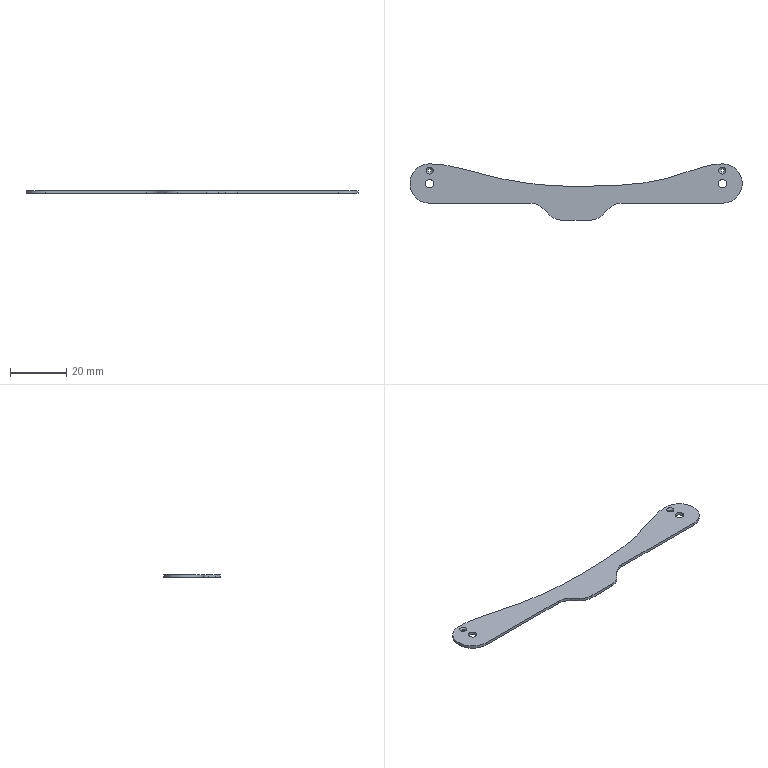Part | NX | features BREP 1, DATUM_CSYS 1, SCALE 1 | 1 solid | 23 faces | box 118 x 20 x 1 mm | volume 1195 mm3 | cylinder 11 | plane 8 | cone 2 | spline 2 | commonest cylinder face diameters 12 x5 1.32 x2 3 x2 14 x2
STEP:
#1=CARTESIAN_POINT('',(-50.74,4.6,1.));
#2=VERTEX_POINT('',#1);
#3=CARTESIAN_POINT('',(-52.,4.6,1.));
#4=DIRECTION('',(0.,0.,1.));
#5=DIRECTION('',(1.,0.,0.));
#6=AXIS2_PLACEMENT_3D('',#3,#4,#5);
#7=CIRCLE('',#6,1.26);
#8=EDGE_CURVE('',#2,#2,#7,.T.);
#9=ORIENTED_EDGE('',*,*,#8,.T.);
#10=EDGE_LOOP('',(#9));
#11=FACE_BOUND('',#10,.T.);
#12=CARTESIAN_POINT('',(-51.34,4.6,0.4));
#13=VERTEX_POINT('',#12);
#14=CARTESIAN_POINT('',(-52.,4.6,0.4));
#15=DIRECTION('',(0.,0.,1.));
#16=DIRECTION('',(1.,0.,0.));
#17=AXIS2_PLACEMENT_3D('',#14,#15,#16);
#18=CIRCLE('',#17,0.66);
#19=EDGE_CURVE('',#13,#13,#18,.T.);
#20=ORIENTED_EDGE('',*,*,#19,.F.);
#21=EDGE_LOOP('',(#20));
#22=FACE_BOUND('',#21,.T.);
#23=CARTESIAN_POINT('',(-52.,4.6,1.));
#24=DIRECTION('',(0.,0.,1.));
#25=DIRECTION('',(1.,0.,0.));
#26=AXIS2_PLACEMENT_3D('',#23,#24,#25);
#27=CONICAL_SURFACE('',#26,1.26,0.7854);
#28=ADVANCED_FACE('',(#11,#22),#27,.F.);
#29=ORIENTED_EDGE('',*,*,#19,.T.);
#30=EDGE_LOOP('',(#29));
#31=FACE_BOUND('',#30,.T.);
#32=CARTESIAN_POINT('',(-51.34,4.6,0.));
#33=VERTEX_POINT('',#32);
#34=CARTESIAN_POINT('',(-52.,4.6,0.));
#35=DIRECTION('',(0.,0.,1.));
#36=DIRECTION('',(1.,0.,0.));
#37=AXIS2_PLACEMENT_3D('',#34,#35,#36);
#38=CIRCLE('',#37,0.66);
#39=EDGE_CURVE('',#33,#33,#38,.T.);
#40=ORIENTED_EDGE('',*,*,#39,.F.);
#41=EDGE_LOOP('',(#40));
#42=FACE_BOUND('',#41,.T.);
#43=CARTESIAN_POINT('',(-52.,4.6,1.));
#44=DIRECTION('',(0.,0.,1.));
#45=DIRECTION('',(1.,0.,0.));
#46=AXIS2_PLACEMENT_3D('',#43,#44,#45);
#47=CYLINDRICAL_SURFACE('',#46,0.66);
#48=ADVANCED_FACE('',(#31,#42),#47,.F.);
#49=CARTESIAN_POINT('',(53.26,4.6,1.));
#50=VERTEX_POINT('',#49);
#51=CARTESIAN_POINT('',(52.,4.6,1.));
#52=DIRECTION('',(0.,0.,1.));
#53=DIRECTION('',(1.,0.,0.));
#54=AXIS2_PLACEMENT_3D('',#51,#52,#53);
#55=CIRCLE('',#54,1.26);
#56=EDGE_CURVE('',#50,#50,#55,.T.);
#57=ORIENTED_EDGE('',*,*,#56,.T.);
#58=EDGE_LOOP('',(#57));
#59=FACE_BOUND('',#58,.T.);
#60=CARTESIAN_POINT('',(52.66,4.6,0.4));
#61=VERTEX_POINT('',#60);
#62=CARTESIAN_POINT('',(52.,4.6,0.4));
#63=DIRECTION('',(0.,0.,1.));
#64=DIRECTION('',(1.,0.,0.));
#65=AXIS2_PLACEMENT_3D('',#62,#63,#64);
#66=CIRCLE('',#65,0.66);
#67=EDGE_CURVE('',#61,#61,#66,.T.);
#68=ORIENTED_EDGE('',*,*,#67,.F.);
#69=EDGE_LOOP('',(#68));
#70=FACE_BOUND('',#69,.T.);
#71=CARTESIAN_POINT('',(52.,4.6,1.));
#72=DIRECTION('',(0.,0.,1.));
#73=DIRECTION('',(1.,0.,0.));
#74=AXIS2_PLACEMENT_3D('',#71,#72,#73);
#75=CONICAL_SURFACE('',#74,1.26,0.7854);
#76=ADVANCED_FACE('',(#59,#70),#75,.F.);
#77=ORIENTED_EDGE('',*,*,#67,.T.);
#78=EDGE_LOOP('',(#77));
#79=FACE_BOUND('',#78,.T.);
#80=CARTESIAN_POINT('',(52.66,4.6,0.));
#81=VERTEX_POINT('',#80);
#82=CARTESIAN_POINT('',(52.,4.6,0.));
#83=DIRECTION('',(0.,0.,1.));
#84=DIRECTION('',(1.,0.,0.));
#85=AXIS2_PLACEMENT_3D('',#82,#83,#84);
#86=CIRCLE('',#85,0.66);
#87=EDGE_CURVE('',#81,#81,#86,.T.);
#88=ORIENTED_EDGE('',*,*,#87,.F.);
#89=EDGE_LOOP('',(#88));
#90=FACE_BOUND('',#89,.T.);
#91=CARTESIAN_POINT('',(52.,4.6,1.));
#92=DIRECTION('',(0.,0.,1.));
#93=DIRECTION('',(1.,0.,0.));
#94=AXIS2_PLACEMENT_3D('',#91,#92,#93);
#95=CYLINDRICAL_SURFACE('',#94,0.66);
#96=ADVANCED_FACE('',(#79,#90),#95,.F.);
#97=CARTESIAN_POINT('',(-50.5,0.,1.));
#98=VERTEX_POINT('',#97);
#99=CARTESIAN_POINT('',(-52.,0.,1.));
#100=DIRECTION('',(0.,0.,1.));
#101=DIRECTION('',(1.,0.,0.));
#102=AXIS2_PLACEMENT_3D('',#99,#100,#101);
#103=CIRCLE('',#102,1.5);
#104=EDGE_CURVE('',#98,#98,#103,.T.);
#105=ORIENTED_EDGE('',*,*,#104,.T.);
#106=EDGE_LOOP('',(#105));
#107=FACE_BOUND('',#106,.T.);
#108=CARTESIAN_POINT('',(-50.5,0.,0.));
#109=VERTEX_POINT('',#108);
#110=CARTESIAN_POINT('',(-52.,0.,0.));
#111=DIRECTION('',(0.,0.,1.));
#112=DIRECTION('',(1.,0.,0.));
#113=AXIS2_PLACEMENT_3D('',#110,#111,#112);
#114=CIRCLE('',#113,1.5);
#115=EDGE_CURVE('',#109,#109,#114,.T.);
#116=ORIENTED_EDGE('',*,*,#115,.F.);
#117=EDGE_LOOP('',(#116));
#118=FACE_BOUND('',#117,.T.);
#119=CARTESIAN_POINT('',(-52.,0.,1.));
#120=DIRECTION('',(0.,0.,1.));
#121=DIRECTION('',(1.,0.,0.));
#122=AXIS2_PLACEMENT_3D('',#119,#120,#121);
#123=CYLINDRICAL_SURFACE('',#122,1.5);
#124=ADVANCED_FACE('',(#107,#118),#123,.F.);
#125=CARTESIAN_POINT('',(53.5,0.,1.));
#126=VERTEX_POINT('',#125);
#127=CARTESIAN_POINT('',(52.,0.,1.));
#128=DIRECTION('',(0.,0.,1.));
#129=DIRECTION('',(1.,0.,0.));
#130=AXIS2_PLACEMENT_3D('',#127,#128,#129);
#131=CIRCLE('',#130,1.5);
#132=EDGE_CURVE('',#126,#126,#131,.T.);
#133=ORIENTED_EDGE('',*,*,#132,.T.);
#134=EDGE_LOOP('',(#133));
#135=FACE_BOUND('',#134,.T.);
#136=CARTESIAN_POINT('',(53.5,0.,0.));
#137=VERTEX_POINT('',#136);
#138=CARTESIAN_POINT('',(52.,0.,0.));
#139=DIRECTION('',(0.,0.,1.));
#140=DIRECTION('',(1.,0.,0.));
#141=AXIS2_PLACEMENT_3D('',#138,#139,#140);
#142=CIRCLE('',#141,1.5);
#143=EDGE_CURVE('',#137,#137,#142,.T.);
#144=ORIENTED_EDGE('',*,*,#143,.F.);
#145=EDGE_LOOP('',(#144));
#146=FACE_BOUND('',#145,.T.);
#147=CARTESIAN_POINT('',(52.,0.,1.));
#148=DIRECTION('',(0.,0.,1.));
#149=DIRECTION('',(1.,0.,0.));
#150=AXIS2_PLACEMENT_3D('',#147,#148,#149);
#151=CYLINDRICAL_SURFACE('',#150,1.5);
#152=ADVANCED_FACE('',(#135,#146),#151,.F.);
#153=CARTESIAN_POINT('',(-52.,7.,1.));
#154=VERTEX_POINT('',#153);
#155=CARTESIAN_POINT('',(-52.,-7.,1.));
#156=VERTEX_POINT('',#155);
#157=CARTESIAN_POINT('',(-52.,0.,1.));
#158=DIRECTION('',(0.,0.,1.));
#159=DIRECTION('',(1.,0.,0.));
#160=AXIS2_PLACEMENT_3D('',#157,#158,#159);
#161=CIRCLE('',#160,7.);
#162=EDGE_CURVE('',#154,#156,#161,.T.);
#163=ORIENTED_EDGE('',*,*,#162,.F.);
#164=CARTESIAN_POINT('',(-52.,7.,0.));
#165=VERTEX_POINT('',#164);
#166=CARTESIAN_POINT('',(-52.,7.,1.));
#167=DIRECTION('',(0.,0.,1.));
#168=VECTOR('',#167,1000.);
#169=LINE('',#166,#168);
#170=EDGE_CURVE('',#165,#154,#169,.T.);
#171=ORIENTED_EDGE('',*,*,#170,.F.);
#172=CARTESIAN_POINT('',(-52.,-7.,0.));
#173=VERTEX_POINT('',#172);
#174=CARTESIAN_POINT('',(-52.,0.,0.));
#175=DIRECTION('',(0.,0.,-1.));
#176=DIRECTION('',(1.,0.,0.));
#177=AXIS2_PLACEMENT_3D('',#174,#175,#176);
#178=CIRCLE('',#177,7.);
#179=EDGE_CURVE('',#173,#165,#178,.T.);
#180=ORIENTED_EDGE('',*,*,#179,.F.);
#181=CARTESIAN_POINT('',(-52.,-7.,1.));
#182=DIRECTION('',(0.,0.,-1.));
#183=VECTOR('',#182,1000.);
#184=LINE('',#181,#183);
#185=EDGE_CURVE('',#156,#173,#184,.T.);
#186=ORIENTED_EDGE('',*,*,#185,.F.);
#187=EDGE_LOOP('',(#163,#171,#180,#186));
#188=FACE_BOUND('',#187,.T.);
#189=CARTESIAN_POINT('',(-52.,0.,1.));
#190=DIRECTION('',(0.,0.,-1.));
#191=DIRECTION('',(-1.,0.,0.));
#192=AXIS2_PLACEMENT_3D('',#189,#190,#191);
#193=CYLINDRICAL_SURFACE('',#192,7.);
#194=ADVANCED_FACE('',(#188),#193,.T.);
#195=CARTESIAN_POINT('',(52.,7.,1.));
#196=VERTEX_POINT('',#195);
#197=CARTESIAN_POINT('',(52.,7.,0.));
#198=VERTEX_POINT('',#197);
#199=CARTESIAN_POINT('',(52.,7.,1.));
#200=DIRECTION('',(0.,0.,-1.));
#201=VECTOR('',#200,1000.);
#202=LINE('',#199,#201);
#203=EDGE_CURVE('',#196,#198,#202,.T.);
#204=ORIENTED_EDGE('',*,*,#203,.F.);
#205=CARTESIAN_POINT('',(52.,-7.,1.));
#206=VERTEX_POINT('',#205);
#207=CARTESIAN_POINT('',(52.,0.,1.));
#208=DIRECTION('',(0.,0.,1.));
#209=DIRECTION('',(1.,0.,0.));
#210=AXIS2_PLACEMENT_3D('',#207,#208,#209);
#211=CIRCLE('',#210,7.);
#212=EDGE_CURVE('',#206,#196,#211,.T.);
#213=ORIENTED_EDGE('',*,*,#212,.F.);
#214=CARTESIAN_POINT('',(52.,-7.,0.));
#215=VERTEX_POINT('',#214);
#216=CARTESIAN_POINT('',(52.,-7.,1.));
#217=DIRECTION('',(0.,0.,1.));
#218=VECTOR('',#217,1000.);
#219=LINE('',#216,#218);
#220=EDGE_CURVE('',#215,#206,#219,.T.);
#221=ORIENTED_EDGE('',*,*,#220,.F.);
#222=CARTESIAN_POINT('',(52.,0.,0.));
#223=DIRECTION('',(0.,0.,-1.));
#224=DIRECTION('',(1.,0.,0.));
#225=AXIS2_PLACEMENT_3D('',#222,#223,#224);
#226=CIRCLE('',#225,7.);
#227=EDGE_CURVE('',#198,#215,#226,.T.);
#228=ORIENTED_EDGE('',*,*,#227,.F.);
#229=EDGE_LOOP('',(#204,#213,#221,#228));
#230=FACE_BOUND('',#229,.T.);
#231=CARTESIAN_POINT('',(52.,0.,1.));
#232=DIRECTION('',(0.,0.,-1.));
#233=DIRECTION('',(-1.,0.,0.));
#234=AXIS2_PLACEMENT_3D('',#231,#232,#233);
#235=CYLINDRICAL_SURFACE('',#234,7.);
#236=ADVANCED_FACE('',(#230),#235,.T.);
#237=CARTESIAN_POINT('',(-15.985,-7.,0.));
#238=VERTEX_POINT('',#237);
#239=CARTESIAN_POINT('',(-59.,-7.,0.));
#240=DIRECTION('',(1.,0.,0.));
#241=VECTOR('',#240,1000.);
#242=LINE('',#239,#241);
#243=EDGE_CURVE('',#173,#238,#242,.T.);
#244=ORIENTED_EDGE('',*,*,#243,.T.);
#245=CARTESIAN_POINT('',(-15.985,-7.,1.));
#246=VERTEX_POINT('',#245);
#247=CARTESIAN_POINT('',(-15.985,-7.,1.));
#248=DIRECTION('',(0.,0.,1.));
#249=VECTOR('',#248,1000.);
#250=LINE('',#247,#249);
#251=EDGE_CURVE('',#238,#246,#250,.T.);
#252=ORIENTED_EDGE('',*,*,#251,.T.);
#253=CARTESIAN_POINT('',(-59.,-7.,1.));
#254=DIRECTION('',(1.,0.,0.));
#255=VECTOR('',#254,1000.);
#256=LINE('',#253,#255);
#257=EDGE_CURVE('',#156,#246,#256,.T.);
#258=ORIENTED_EDGE('',*,*,#257,.F.);
#259=ORIENTED_EDGE('',*,*,#185,.T.);
#260=EDGE_LOOP('',(#244,#252,#258,#259));
#261=FACE_BOUND('',#260,.T.);
#262=CARTESIAN_POINT('',(-59.,-7.,1.));
#263=DIRECTION('',(0.,1.,0.));
#264=DIRECTION('',(0.,0.,1.));
#265=AXIS2_PLACEMENT_3D('',#262,#263,#264);
#266=PLANE('',#265);
#267=ADVANCED_FACE('',(#261),#266,.F.);
#268=CARTESIAN_POINT('',(15.985,-7.,1.));
#269=VERTEX_POINT('',#268);
#270=CARTESIAN_POINT('',(-59.,-7.,1.));
#271=DIRECTION('',(1.,0.,0.));
#272=VECTOR('',#271,1000.);
#273=LINE('',#270,#272);
#274=EDGE_CURVE('',#269,#206,#273,.T.);
#275=ORIENTED_EDGE('',*,*,#274,.F.);
#276=CARTESIAN_POINT('',(15.985,-7.,0.));
#277=VERTEX_POINT('',#276);
#278=CARTESIAN_POINT('',(15.985,-7.,1.));
#279=DIRECTION('',(0.,0.,-1.));
#280=VECTOR('',#279,1000.);
#281=LINE('',#278,#280);
#282=EDGE_CURVE('',#269,#277,#281,.T.);
#283=ORIENTED_EDGE('',*,*,#282,.T.);
#284=CARTESIAN_POINT('',(-59.,-7.,0.));
#285=DIRECTION('',(1.,0.,0.));
#286=VECTOR('',#285,1000.);
#287=LINE('',#284,#286);
#288=EDGE_CURVE('',#277,#215,#287,.T.);
#289=ORIENTED_EDGE('',*,*,#288,.T.);
#290=ORIENTED_EDGE('',*,*,#220,.T.);
#291=EDGE_LOOP('',(#275,#283,#289,#290));
#292=FACE_BOUND('',#291,.T.);
#293=CARTESIAN_POINT('',(-59.,-7.,1.));
#294=DIRECTION('',(0.,1.,0.));
#295=DIRECTION('',(0.,0.,1.));
#296=AXIS2_PLACEMENT_3D('',#293,#294,#295);
#297=PLANE('',#296);
#298=ADVANCED_FACE('',(#292),#297,.F.);
#299=ORIENTED_EDGE('',*,*,#8,.F.);
#300=EDGE_LOOP('',(#299));
#301=FACE_BOUND('',#300,.T.);
#302=ORIENTED_EDGE('',*,*,#56,.F.);
#303=EDGE_LOOP('',(#302));
#304=FACE_BOUND('',#303,.T.);
#305=CARTESIAN_POINT('',(-0.04416,-1.,1.));
#306=VERTEX_POINT('',#305);
#307=CARTESIAN_POINT('',(-52.,7.,1.));
#308=CARTESIAN_POINT('',(-44.778,7.,1.));
#309=CARTESIAN_POINT('',(-28.098,0.9334,1.));
#310=CARTESIAN_POINT('',(-10.53,-1.,1.));
#311=CARTESIAN_POINT('',(-0.04416,-1.,1.));
#312=B_SPLINE_CURVE_WITH_KNOTS('',3,(#307,#308,#309,#310,#311),.UNSPECIFIED.,.F.,.F.,(4,1,4),(0.,0.4049,1.),.UNSPECIFIED.);
#313=EDGE_CURVE('',#154,#306,#312,.T.);
#314=ORIENTED_EDGE('',*,*,#313,.F.);
#315=ORIENTED_EDGE('',*,*,#162,.T.);
#316=ORIENTED_EDGE('',*,*,#257,.T.);
#317=CARTESIAN_POINT('',(-11.743,-8.757,1.));
#318=VERTEX_POINT('',#317);
#319=CARTESIAN_POINT('',(-15.985,-13.,1.));
#320=DIRECTION('',(0.,0.,-1.));
#321=DIRECTION('',(1.,0.,0.));
#322=AXIS2_PLACEMENT_3D('',#319,#320,#321);
#323=CIRCLE('',#322,6.);
#324=EDGE_CURVE('',#246,#318,#323,.T.);
#325=ORIENTED_EDGE('',*,*,#324,.T.);
#326=CARTESIAN_POINT('',(-9.257,-11.243,1.));
#327=VERTEX_POINT('',#326);
#328=CARTESIAN_POINT('',(-10.25,-10.25,1.));
#329=DIRECTION('',(-0.7071,0.7071,0.));
#330=VECTOR('',#329,1000.);
#331=LINE('',#328,#330);
#332=EDGE_CURVE('',#327,#318,#331,.T.);
#333=ORIENTED_EDGE('',*,*,#332,.F.);
#334=CARTESIAN_POINT('',(-5.015,-13.,1.));
#335=VERTEX_POINT('',#334);
#336=CARTESIAN_POINT('',(-5.015,-7.,1.));
#337=DIRECTION('',(0.,0.,1.));
#338=DIRECTION('',(1.,0.,0.));
#339=AXIS2_PLACEMENT_3D('',#336,#337,#338);
#340=CIRCLE('',#339,6.);
#341=EDGE_CURVE('',#327,#335,#340,.T.);
#342=ORIENTED_EDGE('',*,*,#341,.T.);
#343=CARTESIAN_POINT('',(5.015,-13.,1.));
#344=VERTEX_POINT('',#343);
#345=CARTESIAN_POINT('',(0.,-13.,1.));
#346=DIRECTION('',(-1.,0.,0.));
#347=VECTOR('',#346,1000.);
#348=LINE('',#345,#347);
#349=EDGE_CURVE('',#344,#335,#348,.T.);
#350=ORIENTED_EDGE('',*,*,#349,.F.);
#351=CARTESIAN_POINT('',(9.257,-11.243,1.));
#352=VERTEX_POINT('',#351);
#353=CARTESIAN_POINT('',(5.015,-7.,1.));
#354=DIRECTION('',(0.,0.,1.));
#355=DIRECTION('',(1.,0.,0.));
#356=AXIS2_PLACEMENT_3D('',#353,#354,#355);
#357=CIRCLE('',#356,6.);
#358=EDGE_CURVE('',#344,#352,#357,.T.);
#359=ORIENTED_EDGE('',*,*,#358,.T.);
#360=CARTESIAN_POINT('',(11.743,-8.757,1.));
#361=VERTEX_POINT('',#360);
#362=CARTESIAN_POINT('',(10.25,-10.25,1.));
#363=DIRECTION('',(-0.7071,-0.7071,0.));
#364=VECTOR('',#363,1000.);
#365=LINE('',#362,#364);
#366=EDGE_CURVE('',#361,#352,#365,.T.);
#367=ORIENTED_EDGE('',*,*,#366,.F.);
#368=CARTESIAN_POINT('',(15.985,-13.,1.));
#369=DIRECTION('',(0.,0.,-1.));
#370=DIRECTION('',(1.,0.,0.));
#371=AXIS2_PLACEMENT_3D('',#368,#369,#370);
#372=CIRCLE('',#371,6.);
#373=EDGE_CURVE('',#361,#269,#372,.T.);
#374=ORIENTED_EDGE('',*,*,#373,.T.);
#375=ORIENTED_EDGE('',*,*,#274,.T.);
#376=ORIENTED_EDGE('',*,*,#212,.T.);
#377=CARTESIAN_POINT('',(0.05066,-1.,1.));
#378=VERTEX_POINT('',#377);
#379=CARTESIAN_POINT('',(0.05066,-1.,1.));
#380=CARTESIAN_POINT('',(11.936,-0.9991,1.));
#381=CARTESIAN_POINT('',(29.741,-0.7431,1.));
#382=CARTESIAN_POINT('',(46.343,7.,1.));
#383=CARTESIAN_POINT('',(52.,7.,1.));
#384=B_SPLINE_CURVE_WITH_KNOTS('',3,(#379,#380,#381,#382,#383),.UNSPECIFIED.,.F.,.F.,(4,1,4),(0.,0.6757,1.),.UNSPECIFIED.);
#385=EDGE_CURVE('',#378,#196,#384,.T.);
#386=ORIENTED_EDGE('',*,*,#385,.F.);
#387=CARTESIAN_POINT('',(0.04416,-1.,1.));
#388=VERTEX_POINT('',#387);
#389=CARTESIAN_POINT('',(0.04416,5.,1.));
#390=DIRECTION('',(0.,0.,-1.));
#391=DIRECTION('',(1.,0.,0.));
#392=AXIS2_PLACEMENT_3D('',#389,#390,#391);
#393=CIRCLE('',#392,6.);
#394=EDGE_CURVE('',#378,#388,#393,.T.);
#395=ORIENTED_EDGE('',*,*,#394,.T.);
#396=CARTESIAN_POINT('',(0.,-1.,1.));
#397=DIRECTION('',(1.,0.,0.));
#398=VECTOR('',#397,1000.);
#399=LINE('',#396,#398);
#400=EDGE_CURVE('',#306,#388,#399,.T.);
#401=ORIENTED_EDGE('',*,*,#400,.F.);
#402=EDGE_LOOP('',(#314,#315,#316,#325,#333,#342,#350,#359,#367,#374,#375,#376,#386,#395,#401));
#403=FACE_BOUND('',#402,.T.);
#404=ORIENTED_EDGE('',*,*,#104,.F.);
#405=EDGE_LOOP('',(#404));
#406=FACE_BOUND('',#405,.T.);
#407=ORIENTED_EDGE('',*,*,#132,.F.);
#408=EDGE_LOOP('',(#407));
#409=FACE_BOUND('',#408,.T.);
#410=CARTESIAN_POINT('',(0.,0.,1.));
#411=DIRECTION('',(0.,0.,1.));
#412=DIRECTION('',(1.,0.,0.));
#413=AXIS2_PLACEMENT_3D('',#410,#411,#412);
#414=PLANE('',#413);
#415=ADVANCED_FACE('',(#301,#304,#403,#406,#409),#414,.T.);
#416=ORIENTED_EDGE('',*,*,#39,.T.);
#417=EDGE_LOOP('',(#416));
#418=FACE_BOUND('',#417,.T.);
#419=ORIENTED_EDGE('',*,*,#87,.T.);
#420=EDGE_LOOP('',(#419));
#421=FACE_BOUND('',#420,.T.);
#422=ORIENTED_EDGE('',*,*,#115,.T.);
#423=EDGE_LOOP('',(#422));
#424=FACE_BOUND('',#423,.T.);
#425=ORIENTED_EDGE('',*,*,#143,.T.);
#426=EDGE_LOOP('',(#425));
#427=FACE_BOUND('',#426,.T.);
#428=ORIENTED_EDGE('',*,*,#179,.T.);
#429=CARTESIAN_POINT('',(-0.04416,-1.,0.));
#430=VERTEX_POINT('',#429);
#431=CARTESIAN_POINT('',(-52.,7.,0.));
#432=CARTESIAN_POINT('',(-44.778,7.,0.));
#433=CARTESIAN_POINT('',(-28.098,0.9334,0.));
#434=CARTESIAN_POINT('',(-10.53,-1.,0.));
#435=CARTESIAN_POINT('',(-0.04416,-1.,0.));
#436=B_SPLINE_CURVE_WITH_KNOTS('',3,(#431,#432,#433,#434,#435),.UNSPECIFIED.,.F.,.F.,(4,1,4),(0.,0.4049,1.),.UNSPECIFIED.);
#437=EDGE_CURVE('',#165,#430,#436,.T.);
#438=ORIENTED_EDGE('',*,*,#437,.T.);
#439=CARTESIAN_POINT('',(0.04416,-1.,0.));
#440=VERTEX_POINT('',#439);
#441=CARTESIAN_POINT('',(0.,-1.,0.));
#442=DIRECTION('',(-1.,0.,0.));
#443=VECTOR('',#442,1000.);
#444=LINE('',#441,#443);
#445=EDGE_CURVE('',#440,#430,#444,.T.);
#446=ORIENTED_EDGE('',*,*,#445,.F.);
#447=CARTESIAN_POINT('',(0.05066,-1.,0.));
#448=VERTEX_POINT('',#447);
#449=CARTESIAN_POINT('',(0.04416,5.,0.));
#450=DIRECTION('',(0.,0.,1.));
#451=DIRECTION('',(1.,0.,0.));
#452=AXIS2_PLACEMENT_3D('',#449,#450,#451);
#453=CIRCLE('',#452,6.);
#454=EDGE_CURVE('',#440,#448,#453,.T.);
#455=ORIENTED_EDGE('',*,*,#454,.T.);
#456=CARTESIAN_POINT('',(0.05066,-1.,0.));
#457=CARTESIAN_POINT('',(11.936,-0.9991,0.));
#458=CARTESIAN_POINT('',(29.741,-0.7431,0.));
#459=CARTESIAN_POINT('',(46.343,7.,0.));
#460=CARTESIAN_POINT('',(52.,7.,0.));
#461=B_SPLINE_CURVE_WITH_KNOTS('',3,(#456,#457,#458,#459,#460),.UNSPECIFIED.,.F.,.F.,(4,1,4),(0.,0.6757,1.),.UNSPECIFIED.);
#462=EDGE_CURVE('',#448,#198,#461,.T.);
#463=ORIENTED_EDGE('',*,*,#462,.T.);
#464=ORIENTED_EDGE('',*,*,#227,.T.);
#465=ORIENTED_EDGE('',*,*,#288,.F.);
#466=CARTESIAN_POINT('',(11.743,-8.757,0.));
#467=VERTEX_POINT('',#466);
#468=CARTESIAN_POINT('',(15.985,-13.,0.));
#469=DIRECTION('',(0.,0.,1.));
#470=DIRECTION('',(1.,0.,0.));
#471=AXIS2_PLACEMENT_3D('',#468,#469,#470);
#472=CIRCLE('',#471,6.);
#473=EDGE_CURVE('',#277,#467,#472,.T.);
#474=ORIENTED_EDGE('',*,*,#473,.T.);
#475=CARTESIAN_POINT('',(9.257,-11.243,0.));
#476=VERTEX_POINT('',#475);
#477=CARTESIAN_POINT('',(10.25,-10.25,0.));
#478=DIRECTION('',(-0.7071,-0.7071,0.));
#479=VECTOR('',#478,1000.);
#480=LINE('',#477,#479);
#481=EDGE_CURVE('',#467,#476,#480,.T.);
#482=ORIENTED_EDGE('',*,*,#481,.T.);
#483=CARTESIAN_POINT('',(5.015,-13.,0.));
#484=VERTEX_POINT('',#483);
#485=CARTESIAN_POINT('',(5.015,-7.,0.));
#486=DIRECTION('',(0.,0.,-1.));
#487=DIRECTION('',(1.,0.,0.));
#488=AXIS2_PLACEMENT_3D('',#485,#486,#487);
#489=CIRCLE('',#488,6.);
#490=EDGE_CURVE('',#476,#484,#489,.T.);
#491=ORIENTED_EDGE('',*,*,#490,.T.);
#492=CARTESIAN_POINT('',(-5.015,-13.,0.));
#493=VERTEX_POINT('',#492);
#494=CARTESIAN_POINT('',(0.,-13.,0.));
#495=DIRECTION('',(-1.,0.,0.));
#496=VECTOR('',#495,1000.);
#497=LINE('',#494,#496);
#498=EDGE_CURVE('',#484,#493,#497,.T.);
#499=ORIENTED_EDGE('',*,*,#498,.T.);
#500=CARTESIAN_POINT('',(-9.257,-11.243,0.));
#501=VERTEX_POINT('',#500);
#502=CARTESIAN_POINT('',(-5.015,-7.,0.));
#503=DIRECTION('',(0.,0.,-1.));
#504=DIRECTION('',(1.,0.,0.));
#505=AXIS2_PLACEMENT_3D('',#502,#503,#504);
#506=CIRCLE('',#505,6.);
#507=EDGE_CURVE('',#493,#501,#506,.T.);
#508=ORIENTED_EDGE('',*,*,#507,.T.);
#509=CARTESIAN_POINT('',(-11.743,-8.757,0.));
#510=VERTEX_POINT('',#509);
#511=CARTESIAN_POINT('',(-10.25,-10.25,0.));
#512=DIRECTION('',(-0.7071,0.7071,0.));
#513=VECTOR('',#512,1000.);
#514=LINE('',#511,#513);
#515=EDGE_CURVE('',#501,#510,#514,.T.);
#516=ORIENTED_EDGE('',*,*,#515,.T.);
#517=CARTESIAN_POINT('',(-15.985,-13.,0.));
#518=DIRECTION('',(0.,0.,1.));
#519=DIRECTION('',(1.,0.,0.));
#520=AXIS2_PLACEMENT_3D('',#517,#518,#519);
#521=CIRCLE('',#520,6.);
#522=EDGE_CURVE('',#510,#238,#521,.T.);
#523=ORIENTED_EDGE('',*,*,#522,.T.);
#524=ORIENTED_EDGE('',*,*,#243,.F.);
#525=EDGE_LOOP('',(#428,#438,#446,#455,#463,#464,#465,#474,#482,#491,#499,#508,#516,#523,#524));
#526=FACE_BOUND('',#525,.T.);
#527=CARTESIAN_POINT('',(0.,0.,0.));
#528=DIRECTION('',(0.,0.,1.));
#529=DIRECTION('',(1.,0.,0.));
#530=AXIS2_PLACEMENT_3D('',#527,#528,#529);
#531=PLANE('',#530);
#532=ADVANCED_FACE('',(#418,#421,#424,#427,#526),#531,.F.);
#533=ORIENTED_EDGE('',*,*,#332,.T.);
#534=CARTESIAN_POINT('',(-11.743,-8.757,28.659));
#535=DIRECTION('',(0.,0.,-1.));
#536=VECTOR('',#535,1000.);
#537=LINE('',#534,#536);
#538=EDGE_CURVE('',#318,#510,#537,.T.);
#539=ORIENTED_EDGE('',*,*,#538,.T.);
#540=ORIENTED_EDGE('',*,*,#515,.F.);
#541=CARTESIAN_POINT('',(-9.257,-11.243,28.659));
#542=DIRECTION('',(0.,0.,1.));
#543=VECTOR('',#542,1000.);
#544=LINE('',#541,#543);
#545=EDGE_CURVE('',#501,#327,#544,.T.);
#546=ORIENTED_EDGE('',*,*,#545,.T.);
#547=EDGE_LOOP('',(#533,#539,#540,#546));
#548=FACE_BOUND('',#547,.T.);
#549=CARTESIAN_POINT('',(-10.25,-10.25,28.659));
#550=DIRECTION('',(-0.7071,-0.7071,0.));
#551=DIRECTION('',(0.7071,-0.7071,0.));
#552=AXIS2_PLACEMENT_3D('',#549,#550,#551);
#553=PLANE('',#552);
#554=ADVANCED_FACE('',(#548),#553,.T.);
#555=ORIENTED_EDGE('',*,*,#481,.F.);
#556=CARTESIAN_POINT('',(11.743,-8.757,28.659));
#557=DIRECTION('',(0.,0.,1.));
#558=VECTOR('',#557,1000.);
#559=LINE('',#556,#558);
#560=EDGE_CURVE('',#467,#361,#559,.T.);
#561=ORIENTED_EDGE('',*,*,#560,.T.);
#562=ORIENTED_EDGE('',*,*,#366,.T.);
#563=CARTESIAN_POINT('',(9.257,-11.243,28.659));
#564=DIRECTION('',(0.,0.,-1.));
#565=VECTOR('',#564,1000.);
#566=LINE('',#563,#565);
#567=EDGE_CURVE('',#352,#476,#566,.T.);
#568=ORIENTED_EDGE('',*,*,#567,.T.);
#569=EDGE_LOOP('',(#555,#561,#562,#568));
#570=FACE_BOUND('',#569,.T.);
#571=CARTESIAN_POINT('',(10.25,-10.25,28.659));
#572=DIRECTION('',(0.7071,-0.7071,0.));
#573=DIRECTION('',(0.7071,0.7071,0.));
#574=AXIS2_PLACEMENT_3D('',#571,#572,#573);
#575=PLANE('',#574);
#576=ADVANCED_FACE('',(#570),#575,.T.);
#577=ORIENTED_EDGE('',*,*,#498,.F.);
#578=CARTESIAN_POINT('',(5.015,-13.,28.659));
#579=DIRECTION('',(0.,0.,1.));
#580=VECTOR('',#579,1000.);
#581=LINE('',#578,#580);
#582=EDGE_CURVE('',#484,#344,#581,.T.);
#583=ORIENTED_EDGE('',*,*,#582,.T.);
#584=ORIENTED_EDGE('',*,*,#349,.T.);
#585=CARTESIAN_POINT('',(-5.015,-13.,28.659));
#586=DIRECTION('',(0.,0.,-1.));
#587=VECTOR('',#586,1000.);
#588=LINE('',#585,#587);
#589=EDGE_CURVE('',#335,#493,#588,.T.);
#590=ORIENTED_EDGE('',*,*,#589,.T.);
#591=EDGE_LOOP('',(#577,#583,#584,#590));
#592=FACE_BOUND('',#591,.T.);
#593=CARTESIAN_POINT('',(0.,-13.,28.659));
#594=DIRECTION('',(0.,-1.,0.));
#595=DIRECTION('',(0.,0.,-1.));
#596=AXIS2_PLACEMENT_3D('',#593,#594,#595);
#597=PLANE('',#596);
#598=ADVANCED_FACE('',(#592),#597,.T.);
#599=ORIENTED_EDGE('',*,*,#400,.T.);
#600=CARTESIAN_POINT('',(0.04416,-1.,0.));
#601=DIRECTION('',(0.,0.,-1.));
#602=VECTOR('',#601,1000.);
#603=LINE('',#600,#602);
#604=EDGE_CURVE('',#388,#440,#603,.T.);
#605=ORIENTED_EDGE('',*,*,#604,.T.);
#606=ORIENTED_EDGE('',*,*,#445,.T.);
#607=CARTESIAN_POINT('',(-0.04416,-1.,1.));
#608=DIRECTION('',(0.,0.,1.));
#609=VECTOR('',#608,1000.);
#610=LINE('',#607,#609);
#611=EDGE_CURVE('',#430,#306,#610,.T.);
#612=ORIENTED_EDGE('',*,*,#611,.T.);
#613=EDGE_LOOP('',(#599,#605,#606,#612));
#614=FACE_BOUND('',#613,.T.);
#615=CARTESIAN_POINT('',(0.,-1.,2.));
#616=DIRECTION('',(0.,-1.,0.));
#617=DIRECTION('',(0.,0.,-1.));
#618=AXIS2_PLACEMENT_3D('',#615,#616,#617);
#619=PLANE('',#618);
#620=ADVANCED_FACE('',(#614),#619,.F.);
#621=ORIENTED_EDGE('',*,*,#394,.F.);
#622=CARTESIAN_POINT('',(0.05066,-1.,-1.));
#623=DIRECTION('',(0.,0.,-1.));
#624=VECTOR('',#623,1000.);
#625=LINE('',#622,#624);
#626=EDGE_CURVE('',#378,#448,#625,.T.);
#627=ORIENTED_EDGE('',*,*,#626,.T.);
#628=ORIENTED_EDGE('',*,*,#454,.F.);
#629=ORIENTED_EDGE('',*,*,#604,.F.);
#630=EDGE_LOOP('',(#621,#627,#628,#629));
#631=FACE_BOUND('',#630,.T.);
#632=CARTESIAN_POINT('',(0.04416,5.,2.));
#633=DIRECTION('',(0.,0.,1.));
#634=DIRECTION('',(1.,0.,0.));
#635=AXIS2_PLACEMENT_3D('',#632,#633,#634);
#636=CYLINDRICAL_SURFACE('',#635,6.);
#637=ADVANCED_FACE('',(#631),#636,.F.);
#638=ORIENTED_EDGE('',*,*,#324,.F.);
#639=ORIENTED_EDGE('',*,*,#251,.F.);
#640=ORIENTED_EDGE('',*,*,#522,.F.);
#641=ORIENTED_EDGE('',*,*,#538,.F.);
#642=EDGE_LOOP('',(#638,#639,#640,#641));
#643=FACE_BOUND('',#642,.T.);
#644=CARTESIAN_POINT('',(-15.985,-13.,28.659));
#645=DIRECTION('',(0.,0.,-1.));
#646=DIRECTION('',(-1.,0.,0.));
#647=AXIS2_PLACEMENT_3D('',#644,#645,#646);
#648=CYLINDRICAL_SURFACE('',#647,6.);
#649=ADVANCED_FACE('',(#643),#648,.F.);
#650=ORIENTED_EDGE('',*,*,#373,.F.);
#651=ORIENTED_EDGE('',*,*,#560,.F.);
#652=ORIENTED_EDGE('',*,*,#473,.F.);
#653=ORIENTED_EDGE('',*,*,#282,.F.);
#654=EDGE_LOOP('',(#650,#651,#652,#653));
#655=FACE_BOUND('',#654,.T.);
#656=CARTESIAN_POINT('',(15.985,-13.,1.));
#657=DIRECTION('',(0.,0.,-1.));
#658=DIRECTION('',(-1.,0.,0.));
#659=AXIS2_PLACEMENT_3D('',#656,#657,#658);
#660=CYLINDRICAL_SURFACE('',#659,6.);
#661=ADVANCED_FACE('',(#655),#660,.F.);
#662=ORIENTED_EDGE('',*,*,#358,.F.);
#663=ORIENTED_EDGE('',*,*,#582,.F.);
#664=ORIENTED_EDGE('',*,*,#490,.F.);
#665=ORIENTED_EDGE('',*,*,#567,.F.);
#666=EDGE_LOOP('',(#662,#663,#664,#665));
#667=FACE_BOUND('',#666,.T.);
#668=CARTESIAN_POINT('',(5.015,-7.,28.659));
#669=DIRECTION('',(0.,0.,-1.));
#670=DIRECTION('',(-1.,0.,0.));
#671=AXIS2_PLACEMENT_3D('',#668,#669,#670);
#672=CYLINDRICAL_SURFACE('',#671,6.);
#673=ADVANCED_FACE('',(#667),#672,.T.);
#674=ORIENTED_EDGE('',*,*,#341,.F.);
#675=ORIENTED_EDGE('',*,*,#545,.F.);
#676=ORIENTED_EDGE('',*,*,#507,.F.);
#677=ORIENTED_EDGE('',*,*,#589,.F.);
#678=EDGE_LOOP('',(#674,#675,#676,#677));
#679=FACE_BOUND('',#678,.T.);
#680=CARTESIAN_POINT('',(-5.015,-7.,28.659));
#681=DIRECTION('',(0.,0.,-1.));
#682=DIRECTION('',(-1.,0.,0.));
#683=AXIS2_PLACEMENT_3D('',#680,#681,#682);
#684=CYLINDRICAL_SURFACE('',#683,6.);
#685=ADVANCED_FACE('',(#679),#684,.T.);
#686=ORIENTED_EDGE('',*,*,#170,.T.);
#687=ORIENTED_EDGE('',*,*,#313,.T.);
#688=ORIENTED_EDGE('',*,*,#611,.F.);
#689=ORIENTED_EDGE('',*,*,#437,.F.);
#690=EDGE_LOOP('',(#686,#687,#688,#689));
#691=FACE_BOUND('',#690,.T.);
#692=CARTESIAN_POINT('',(-52.,7.,0.));
#693=CARTESIAN_POINT('',(-52.,7.,1.));
#694=CARTESIAN_POINT('',(-44.778,7.,0.));
#695=CARTESIAN_POINT('',(-44.778,7.,1.));
#696=CARTESIAN_POINT('',(-28.098,0.9334,0.));
#697=CARTESIAN_POINT('',(-28.098,0.9334,1.));
#698=CARTESIAN_POINT('',(-10.53,-1.,0.));
#699=CARTESIAN_POINT('',(-10.53,-1.,1.));
#700=CARTESIAN_POINT('',(-0.04416,-1.,0.));
#701=CARTESIAN_POINT('',(-0.04416,-1.,1.));
#702=B_SPLINE_SURFACE_WITH_KNOTS('',3,1,((#692,#693),(#694,#695),(#696,#697),(#698,#699),(#700,#701)),.SURF_OF_LINEAR_EXTRUSION.,.F.,.F.,.F.,(4,1,4),(2,2),(0.,0.4049,1.),(0.,1.),.UNSPECIFIED.);
#703=ADVANCED_FACE('',(#691),#702,.F.);
#704=ORIENTED_EDGE('',*,*,#626,.F.);
#705=ORIENTED_EDGE('',*,*,#385,.T.);
#706=ORIENTED_EDGE('',*,*,#203,.T.);
#707=ORIENTED_EDGE('',*,*,#462,.F.);
#708=EDGE_LOOP('',(#704,#705,#706,#707));
#709=FACE_BOUND('',#708,.T.);
#710=CARTESIAN_POINT('',(0.05066,-1.,0.));
#711=CARTESIAN_POINT('',(0.05066,-1.,1.));
#712=CARTESIAN_POINT('',(11.936,-0.9991,0.));
#713=CARTESIAN_POINT('',(11.936,-0.9991,1.));
#714=CARTESIAN_POINT('',(29.741,-0.7431,0.));
#715=CARTESIAN_POINT('',(29.741,-0.7431,1.));
#716=CARTESIAN_POINT('',(46.343,7.,0.));
#717=CARTESIAN_POINT('',(46.343,7.,1.));
#718=CARTESIAN_POINT('',(52.,7.,0.));
#719=CARTESIAN_POINT('',(52.,7.,1.));
#720=B_SPLINE_SURFACE_WITH_KNOTS('',3,1,((#710,#711),(#712,#713),(#714,#715),(#716,#717),(#718,#719)),.SURF_OF_LINEAR_EXTRUSION.,.F.,.F.,.F.,(4,1,4),(2,2),(0.,0.6757,1.),(0.,1.),.UNSPECIFIED.);
#721=ADVANCED_FACE('',(#709),#720,.F.);
#722=CLOSED_SHELL('',(#28,#48,#76,#96,#124,#152,#194,#236,#267,#298,#415,#532,#554,#576,#598,#620,#637,#649,#661,#673,#685,#703,#721));
#723=MANIFOLD_SOLID_BREP('',#722);
#724=(LENGTH_UNIT()NAMED_UNIT(*)SI_UNIT(.MILLI.,.METRE.));
#725=UNCERTAINTY_MEASURE_WITH_UNIT(LENGTH_MEASURE(0.00001),#724,'','');
#726=(NAMED_UNIT(*)PLANE_ANGLE_UNIT()SI_UNIT($,.RADIAN.));
#727=(NAMED_UNIT(*)SI_UNIT($,.STERADIAN.)SOLID_ANGLE_UNIT());
#728=(GEOMETRIC_REPRESENTATION_CONTEXT(3)GLOBAL_UNCERTAINTY_ASSIGNED_CONTEXT((#725))GLOBAL_UNIT_ASSIGNED_CONTEXT((#724,#726,#727))REPRESENTATION_CONTEXT('',''));
#729=ADVANCED_BREP_SHAPE_REPRESENTATION('',(#723),#728);